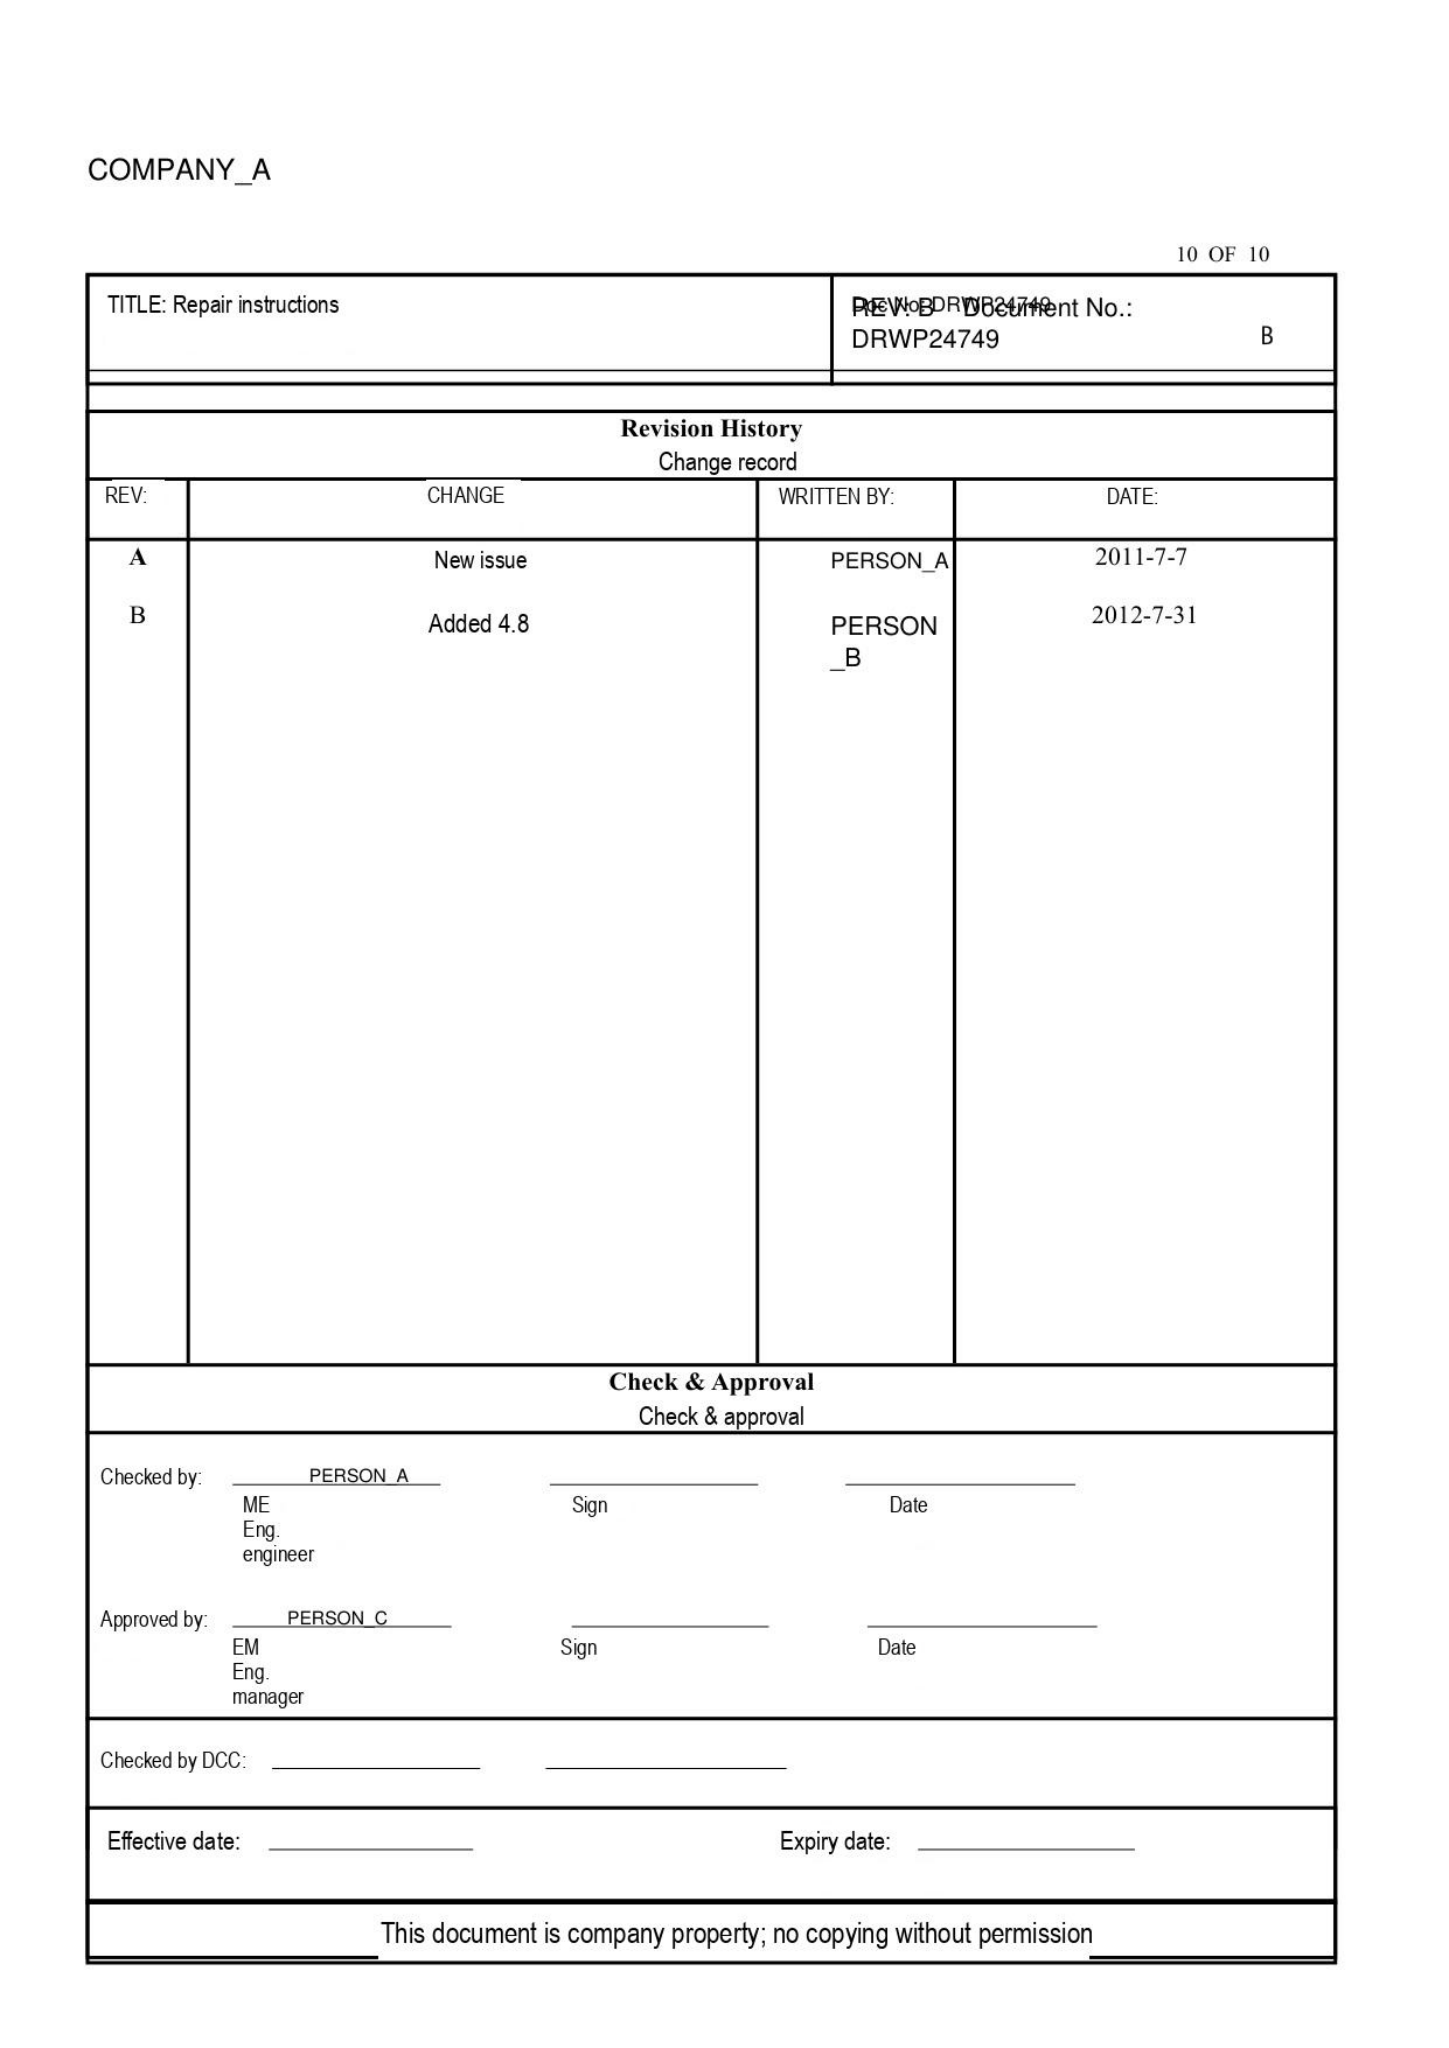COMPANY_A

10 OF 10

| TITLE: Repair instructions | REV: B Document No.: DRWP24749 B |
|---|---|

**Revision History**
Change record

| REV: | CHANGE | WRITTEN BY: | DATE: |
|---|---|---|---|
| A | New issue | PERSON_A | 2011-7-7 |
| B | Added 4.8 | PERSON_B | 2012-7-31 |

**Check & Approval**
Check & approval

Checked by: PERSON_A
ME
Eng.
engineer
Sign
Date

Approved by: PERSON_C
EM
Eng.
manager
Sign
Date

Checked by DCC:

Effective date:
Expiry date:

This document is company property; no copying without permission
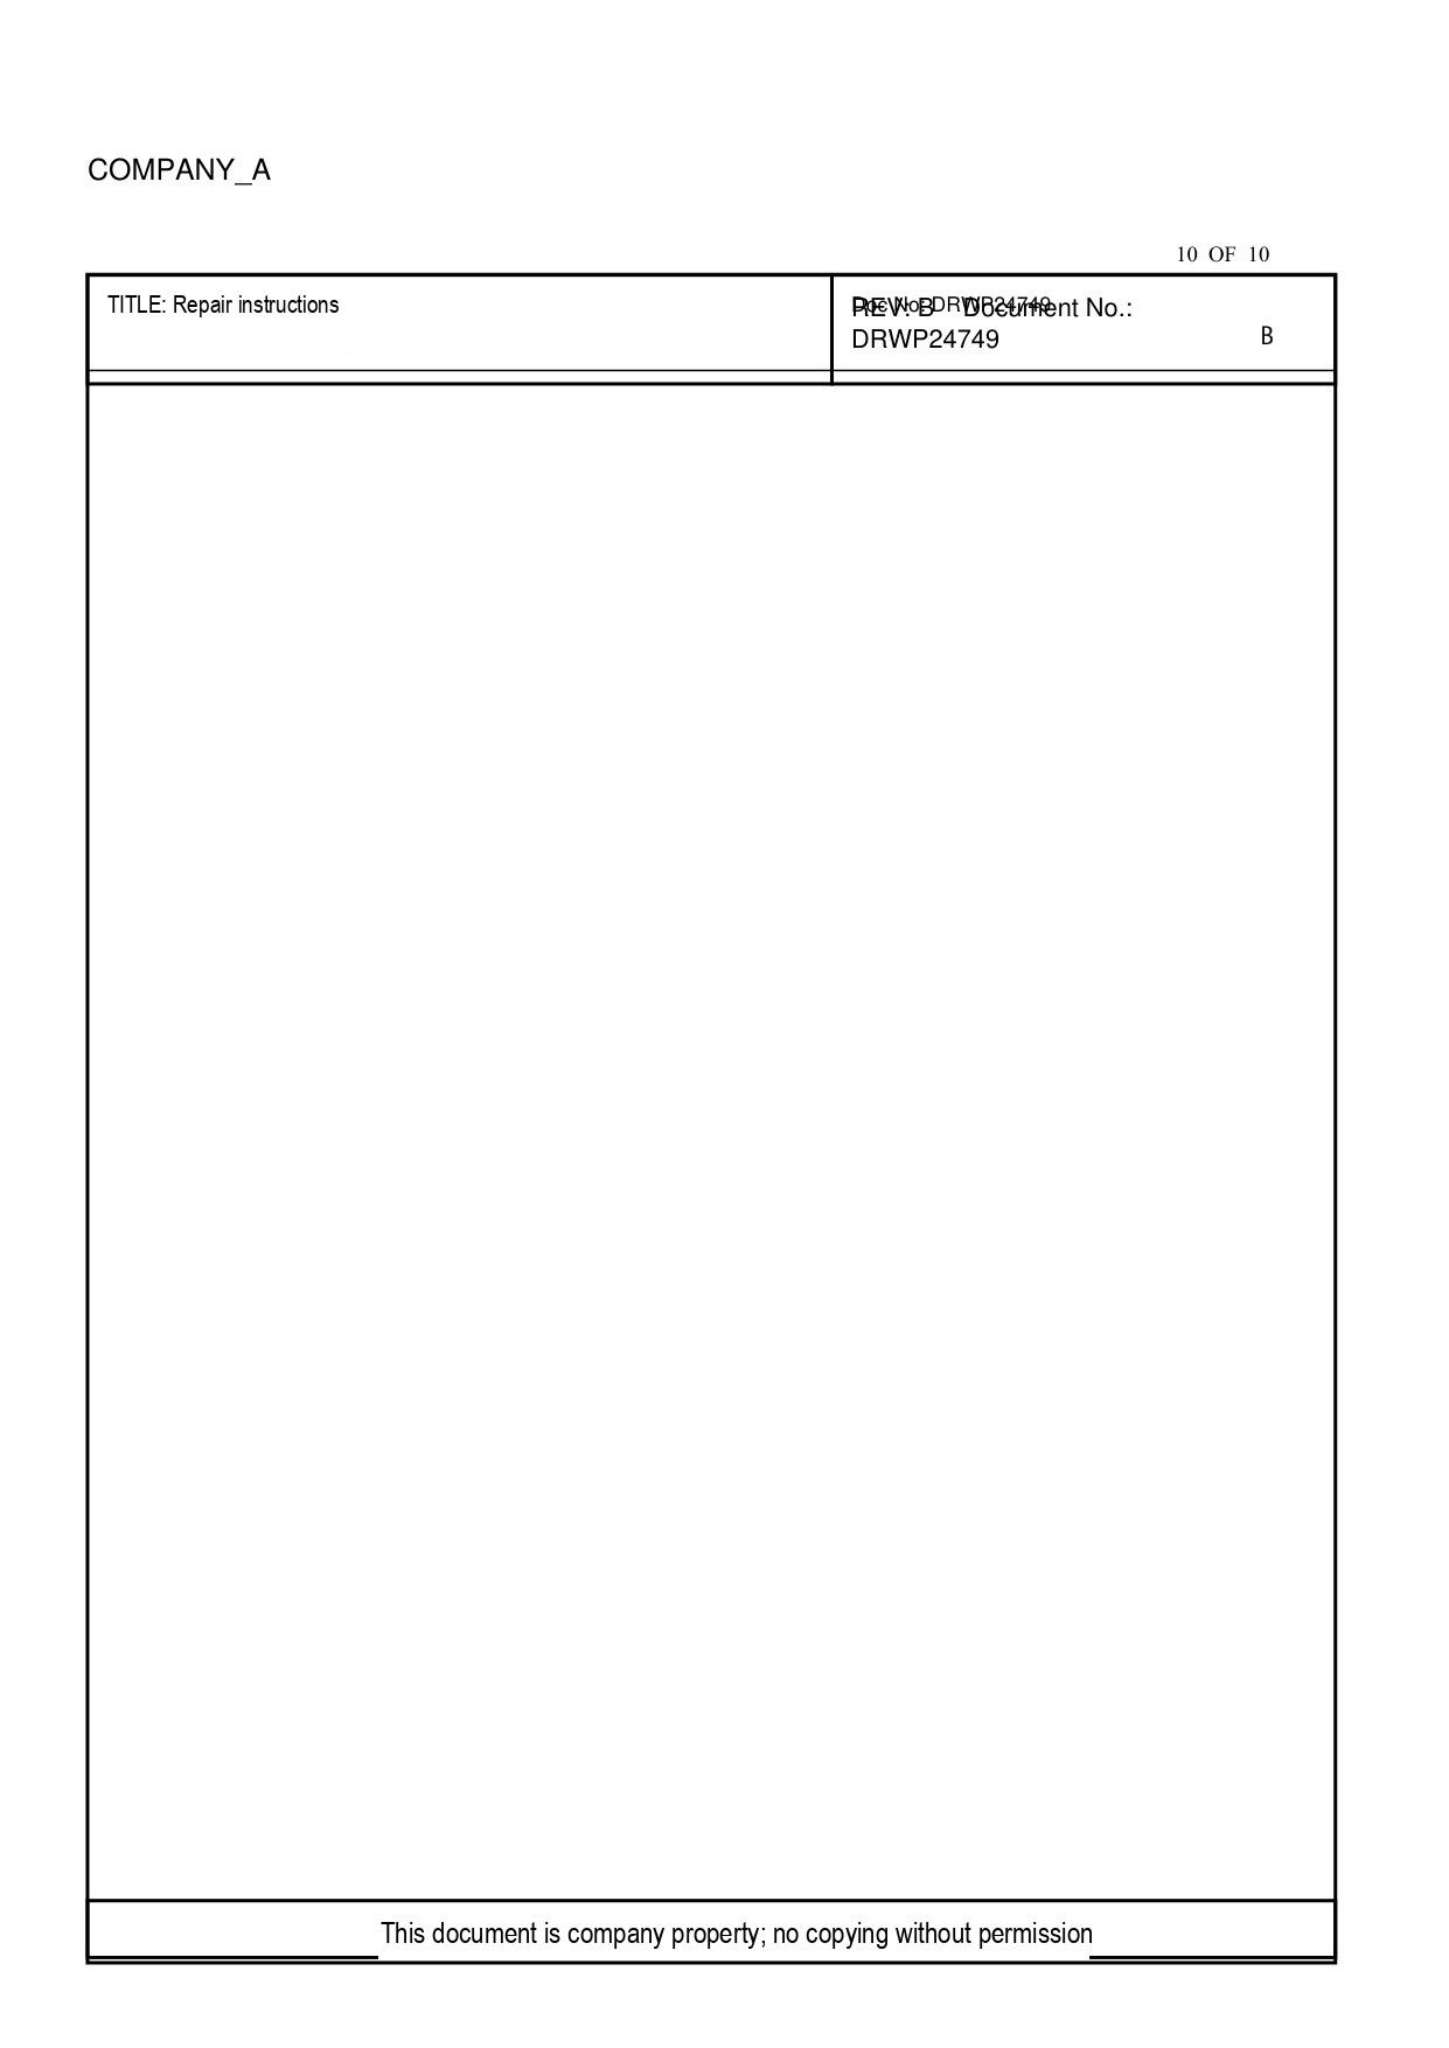COMPANY_A

10 OF 10

| TITLE: Repair instructions | REV: B Document No.: DRWP24749 B |
|---|---|

This document is company property; no copying without permission
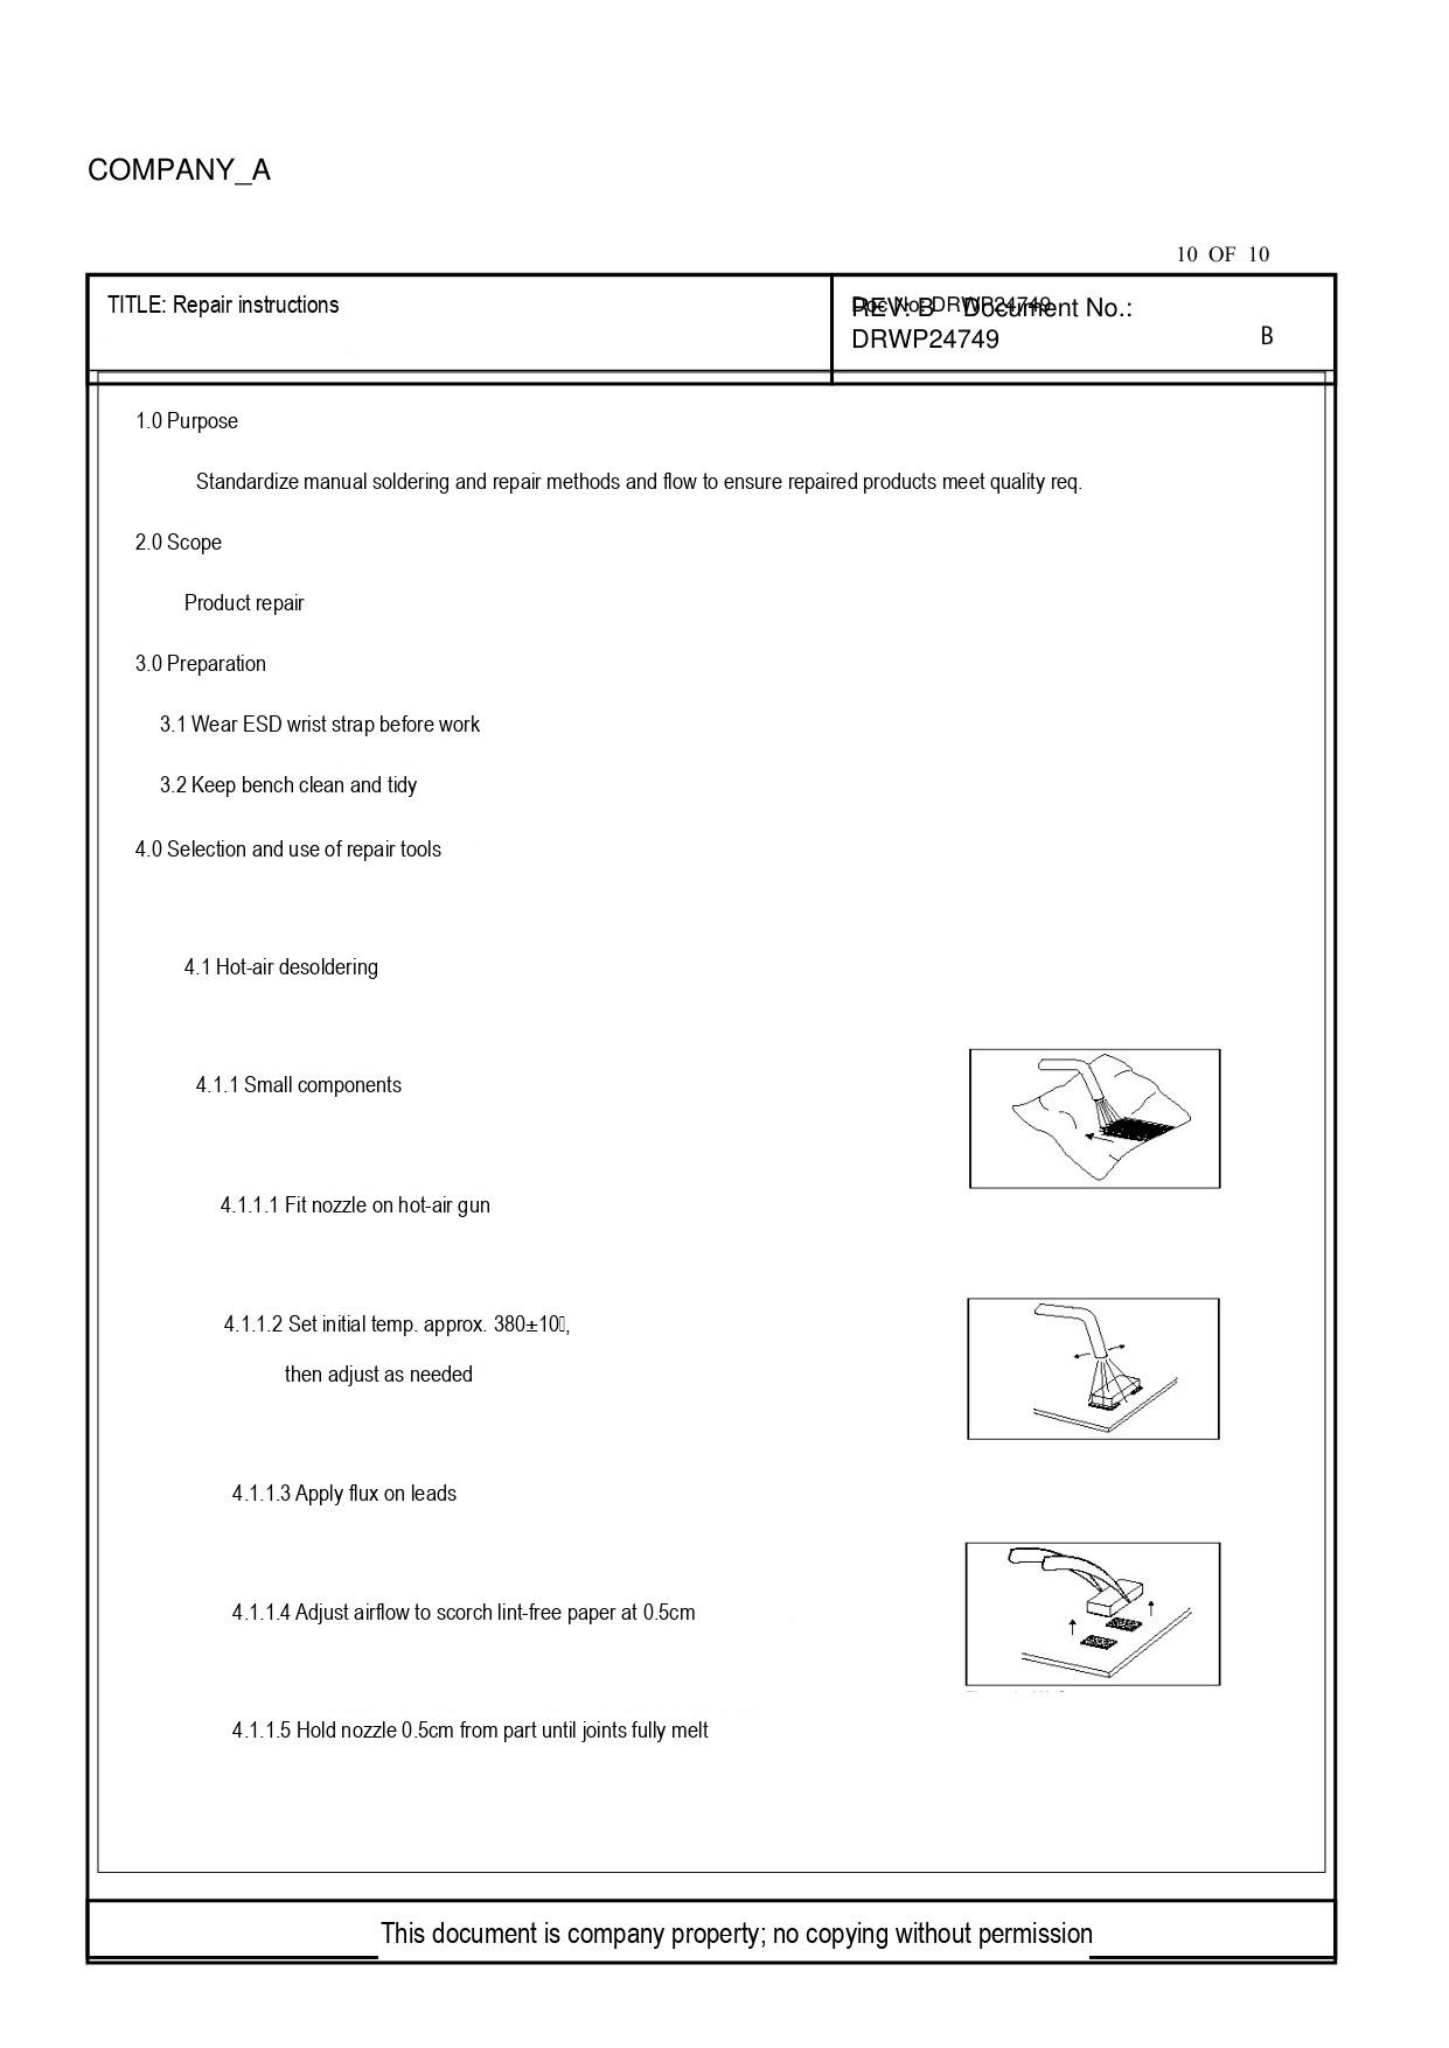COMPANY_A

10 OF 10

| TITLE: Repair instructions | REV: B Document No.: DRWP24749 B |
|---|---|

1.0 Purpose

Standardize manual soldering and repair methods and flow to ensure repaired products meet quality req.

2.0 Scope

Product repair

3.0 Preparation

3.1 Wear ESD wrist strap before work

3.2 Keep bench clean and tidy

4.0 Selection and use of repair tools

4.1 Hot-air desoldering

4.1.1 Small components

4.1.1.1 Fit nozzle on hot-air gun

4.1.1.2 Set initial temp. approx. 380±10,

then adjust as needed

4.1.1.3 Apply flux on leads

4.1.1.4 Adjust airflow to scorch lint-free paper at 0.5cm

4.1.1.5 Hold nozzle 0.5cm from part until joints fully melt

This document is company property; no copying without permission
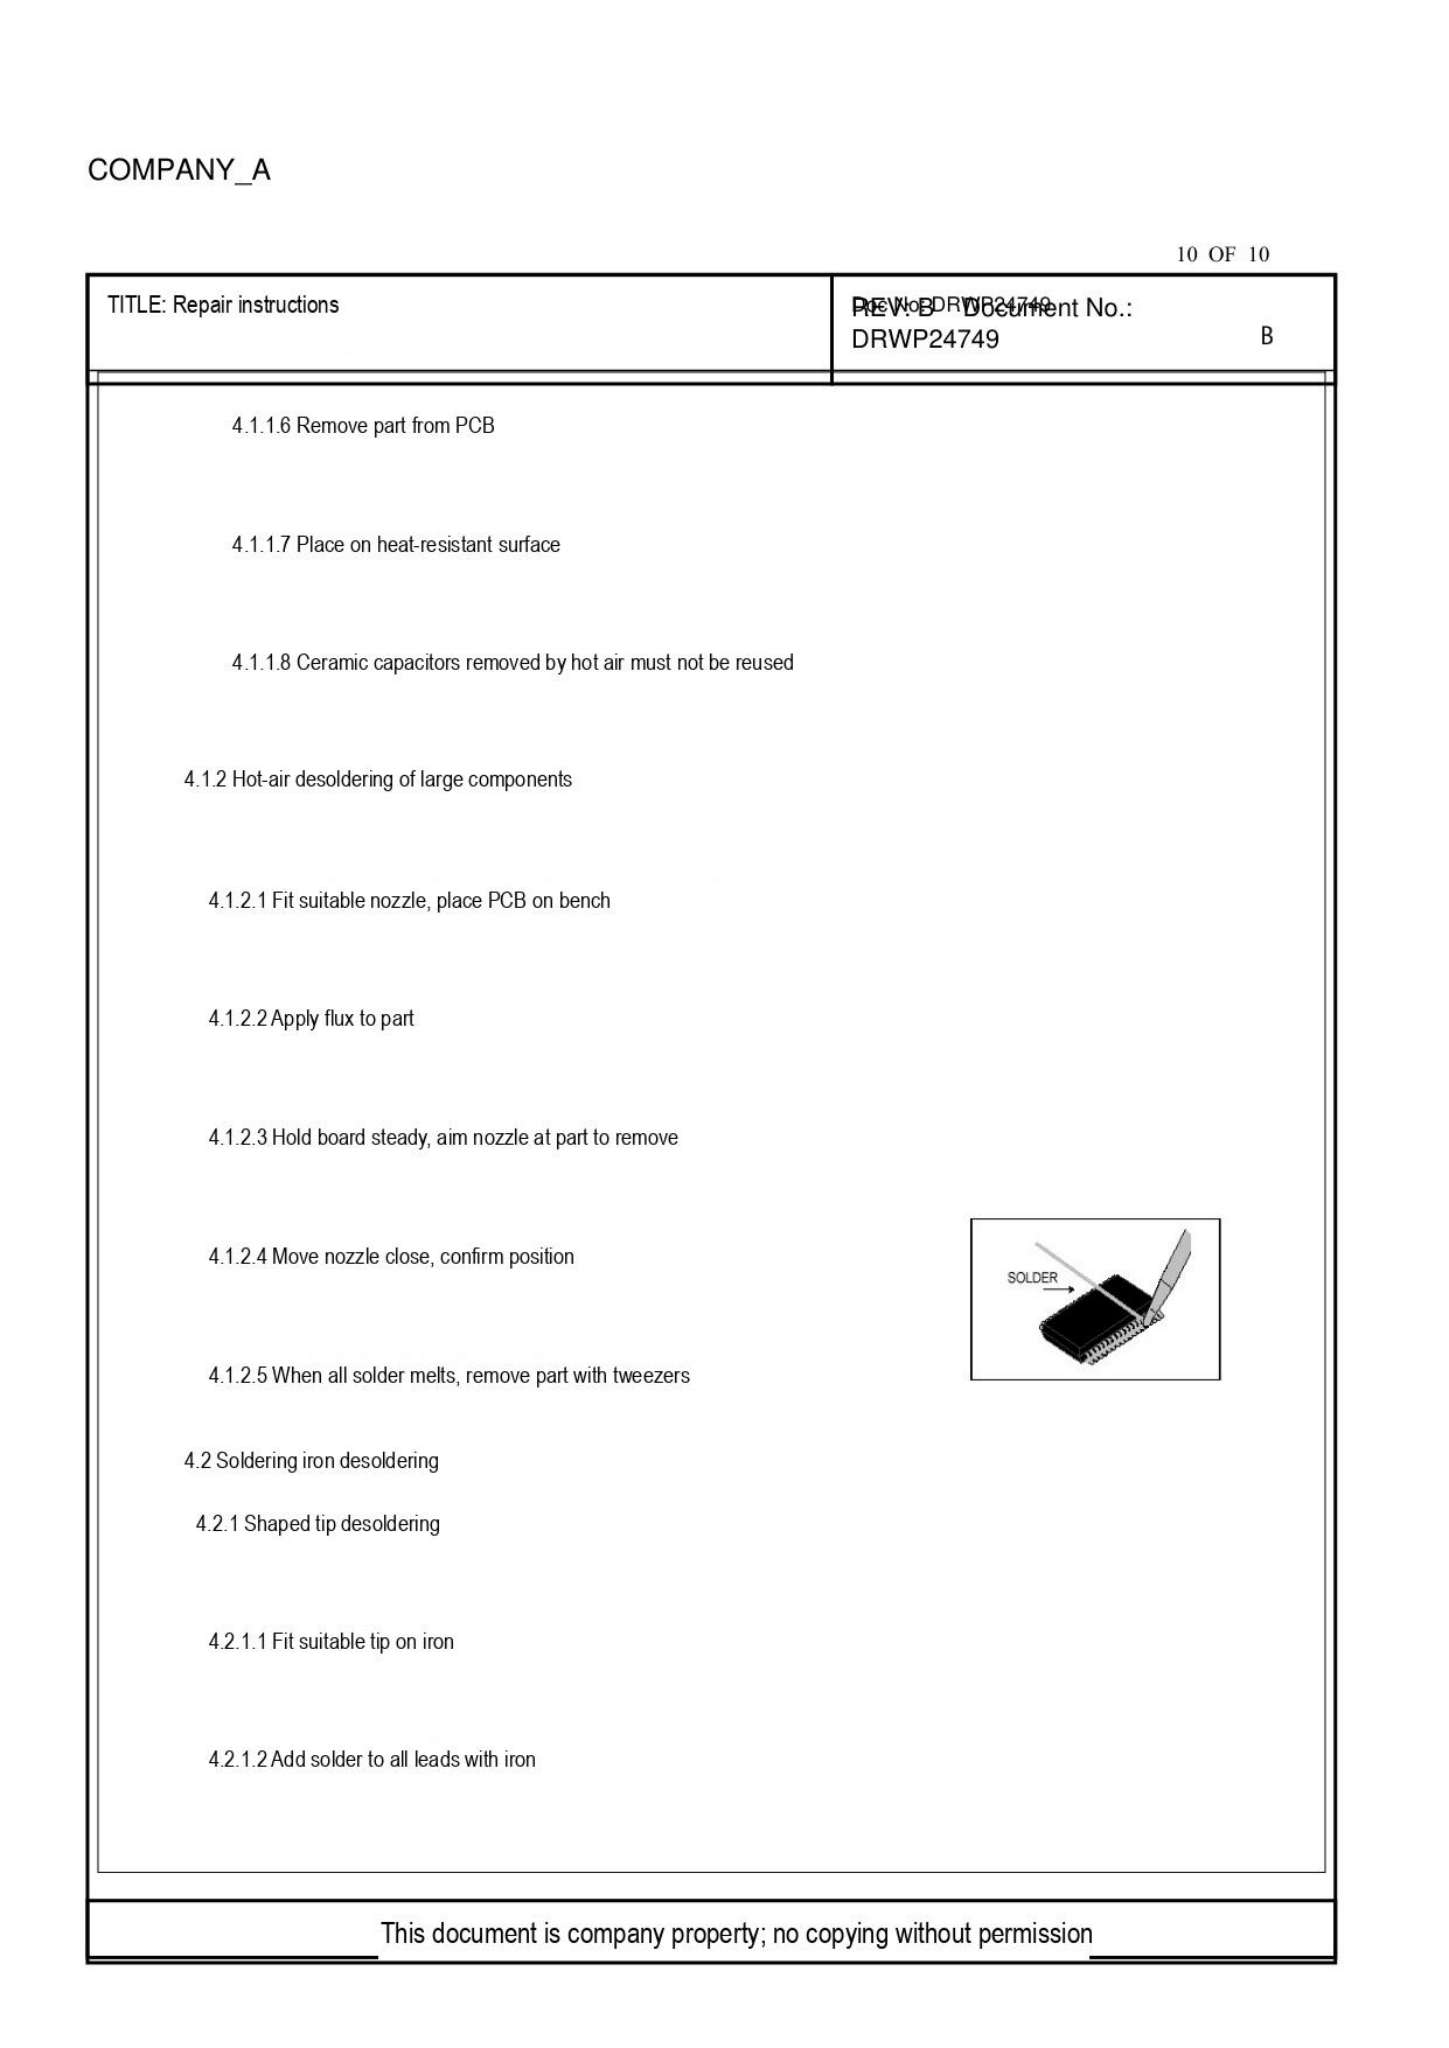COMPANY_A

10 OF 10

| TITLE: Repair instructions | REV: B Document No.: DRWP24749 B |
|---|---|

4.1.1.6 Remove part from PCB

4.1.1.7 Place on heat-resistant surface

4.1.1.8 Ceramic capacitors removed by hot air must not be reused

4.1.2 Hot-air desoldering of large components

4.1.2.1 Fit suitable nozzle, place PCB on bench

4.1.2.2 Apply flux to part

4.1.2.3 Hold board steady, aim nozzle at part to remove

4.1.2.4 Move nozzle close, confirm position

SOLDER

4.1.2.5 When all solder melts, remove part with tweezers

4.2 Soldering iron desoldering

4.2.1 Shaped tip desoldering

4.2.1.1 Fit suitable tip on iron

4.2.1.2 Add solder to all leads with iron

This document is company property; no copying without permission
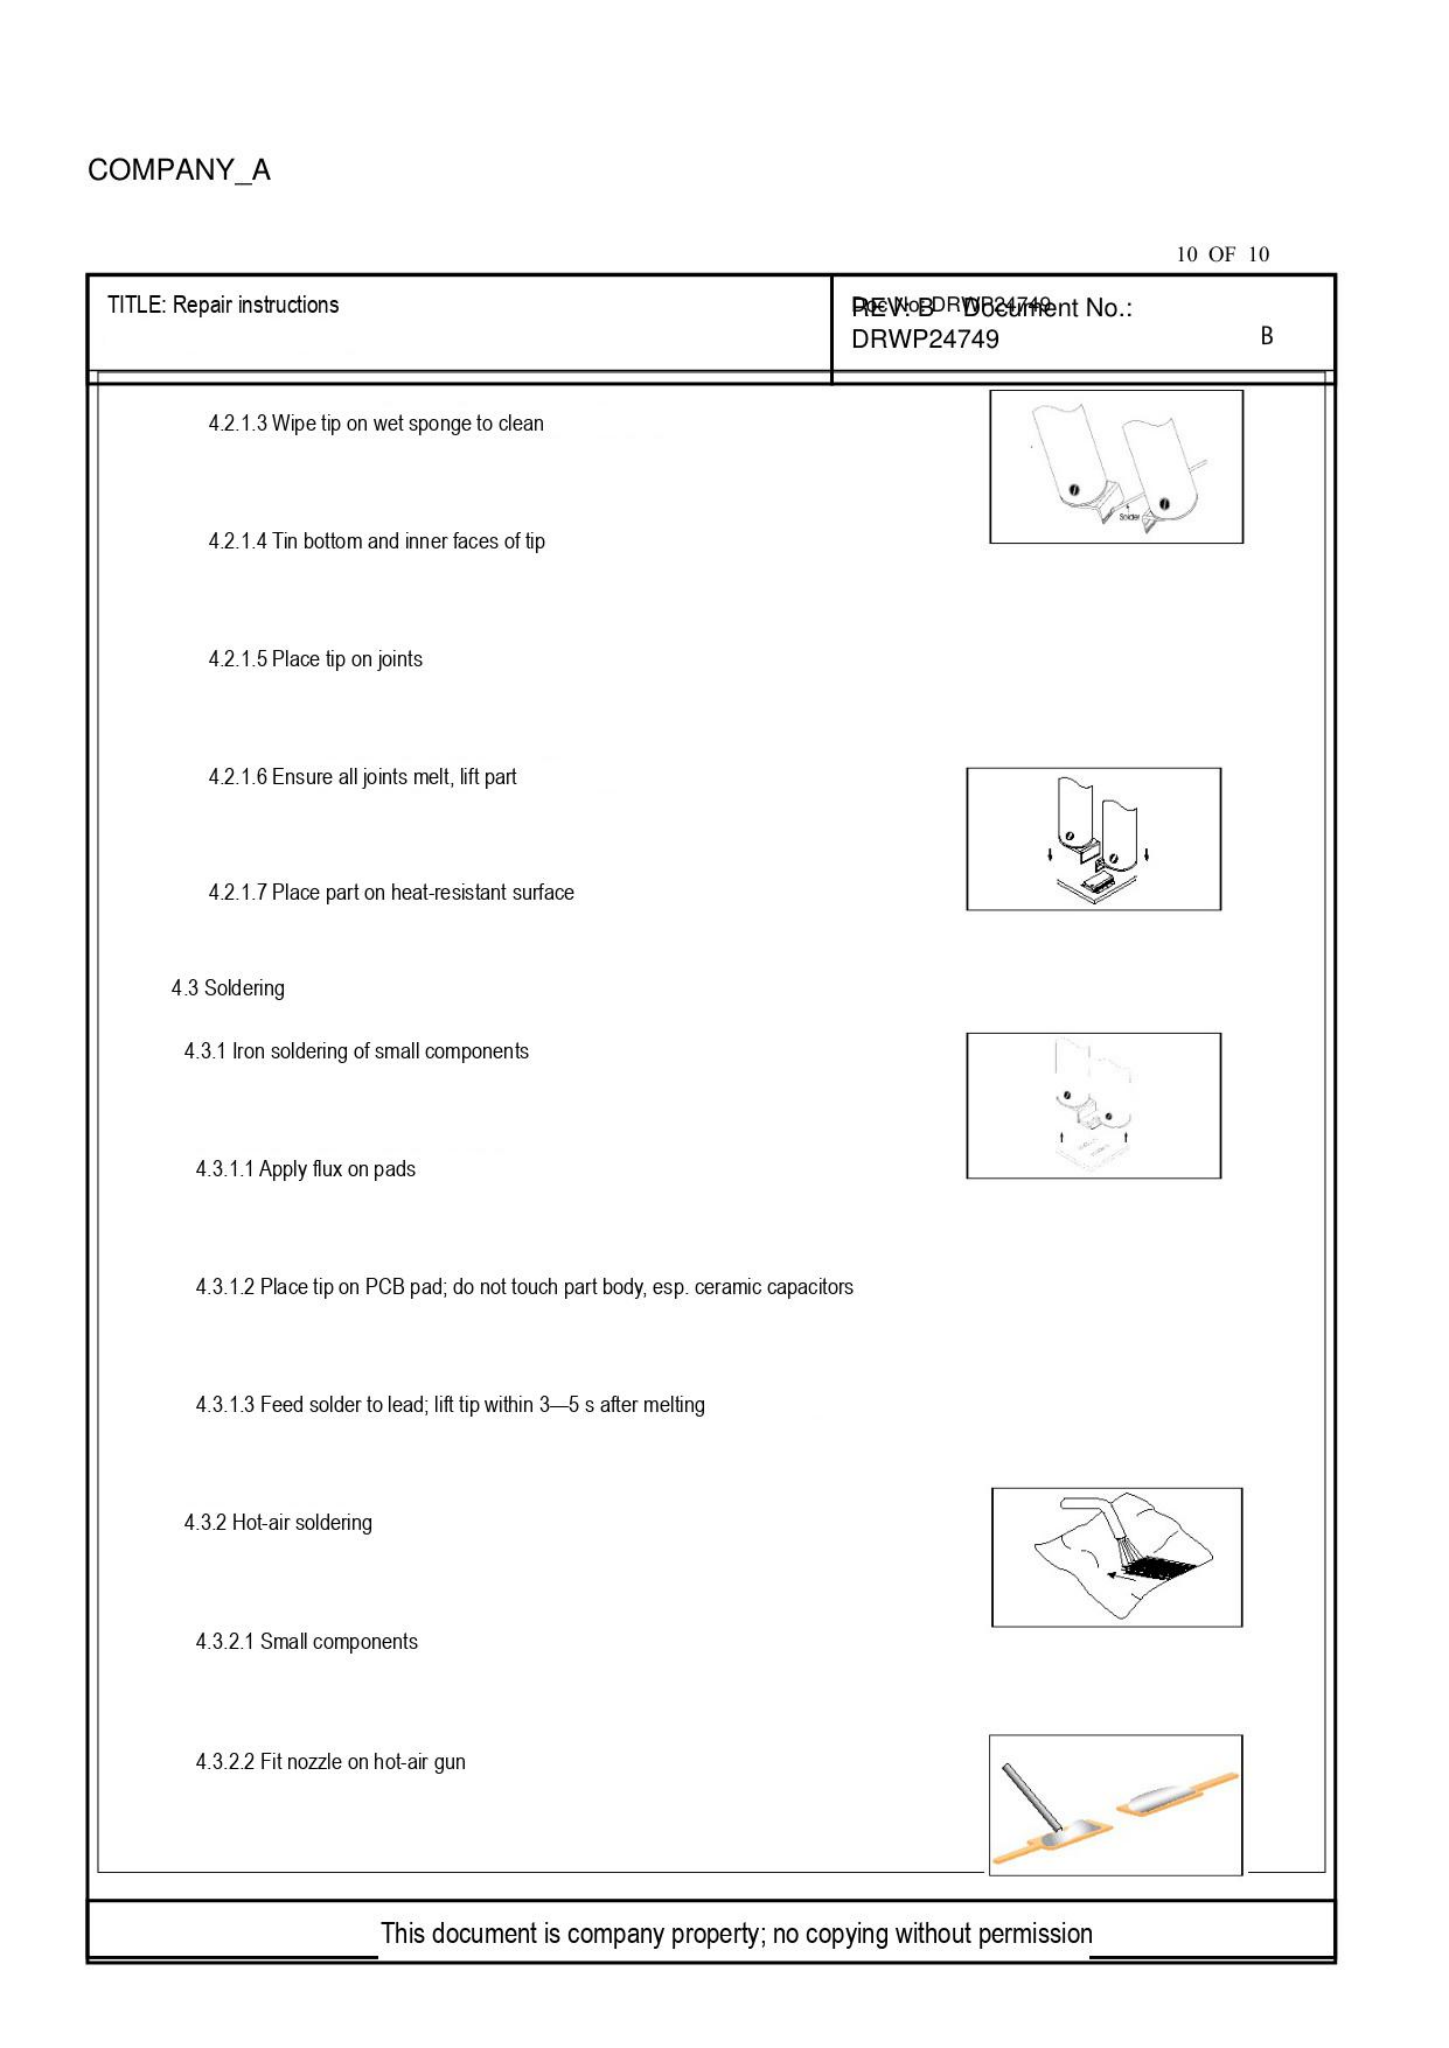COMPANY_A

10 OF 10

| TITLE: Repair instructions | Document No.: DRWP24749 REV: B |
|---|---|

4.2.1.3 Wipe tip on wet sponge to clean

Solder

4.2.1.4 Tin bottom and inner faces of tip

4.2.1.5 Place tip on joints

4.2.1.6 Ensure all joints melt, lift part

4.2.1.7 Place part on heat-resistant surface

4.3 Soldering

4.3.1 Iron soldering of small components

4.3.1.1 Apply flux on pads

4.3.1.2 Place tip on PCB pad; do not touch part body, esp. ceramic capacitors

4.3.1.3 Feed solder to lead; lift tip within 3—5 s after melting

4.3.2 Hot-air soldering

4.3.2.1 Small components

4.3.2.2 Fit nozzle on hot-air gun

This document is company property; no copying without permission
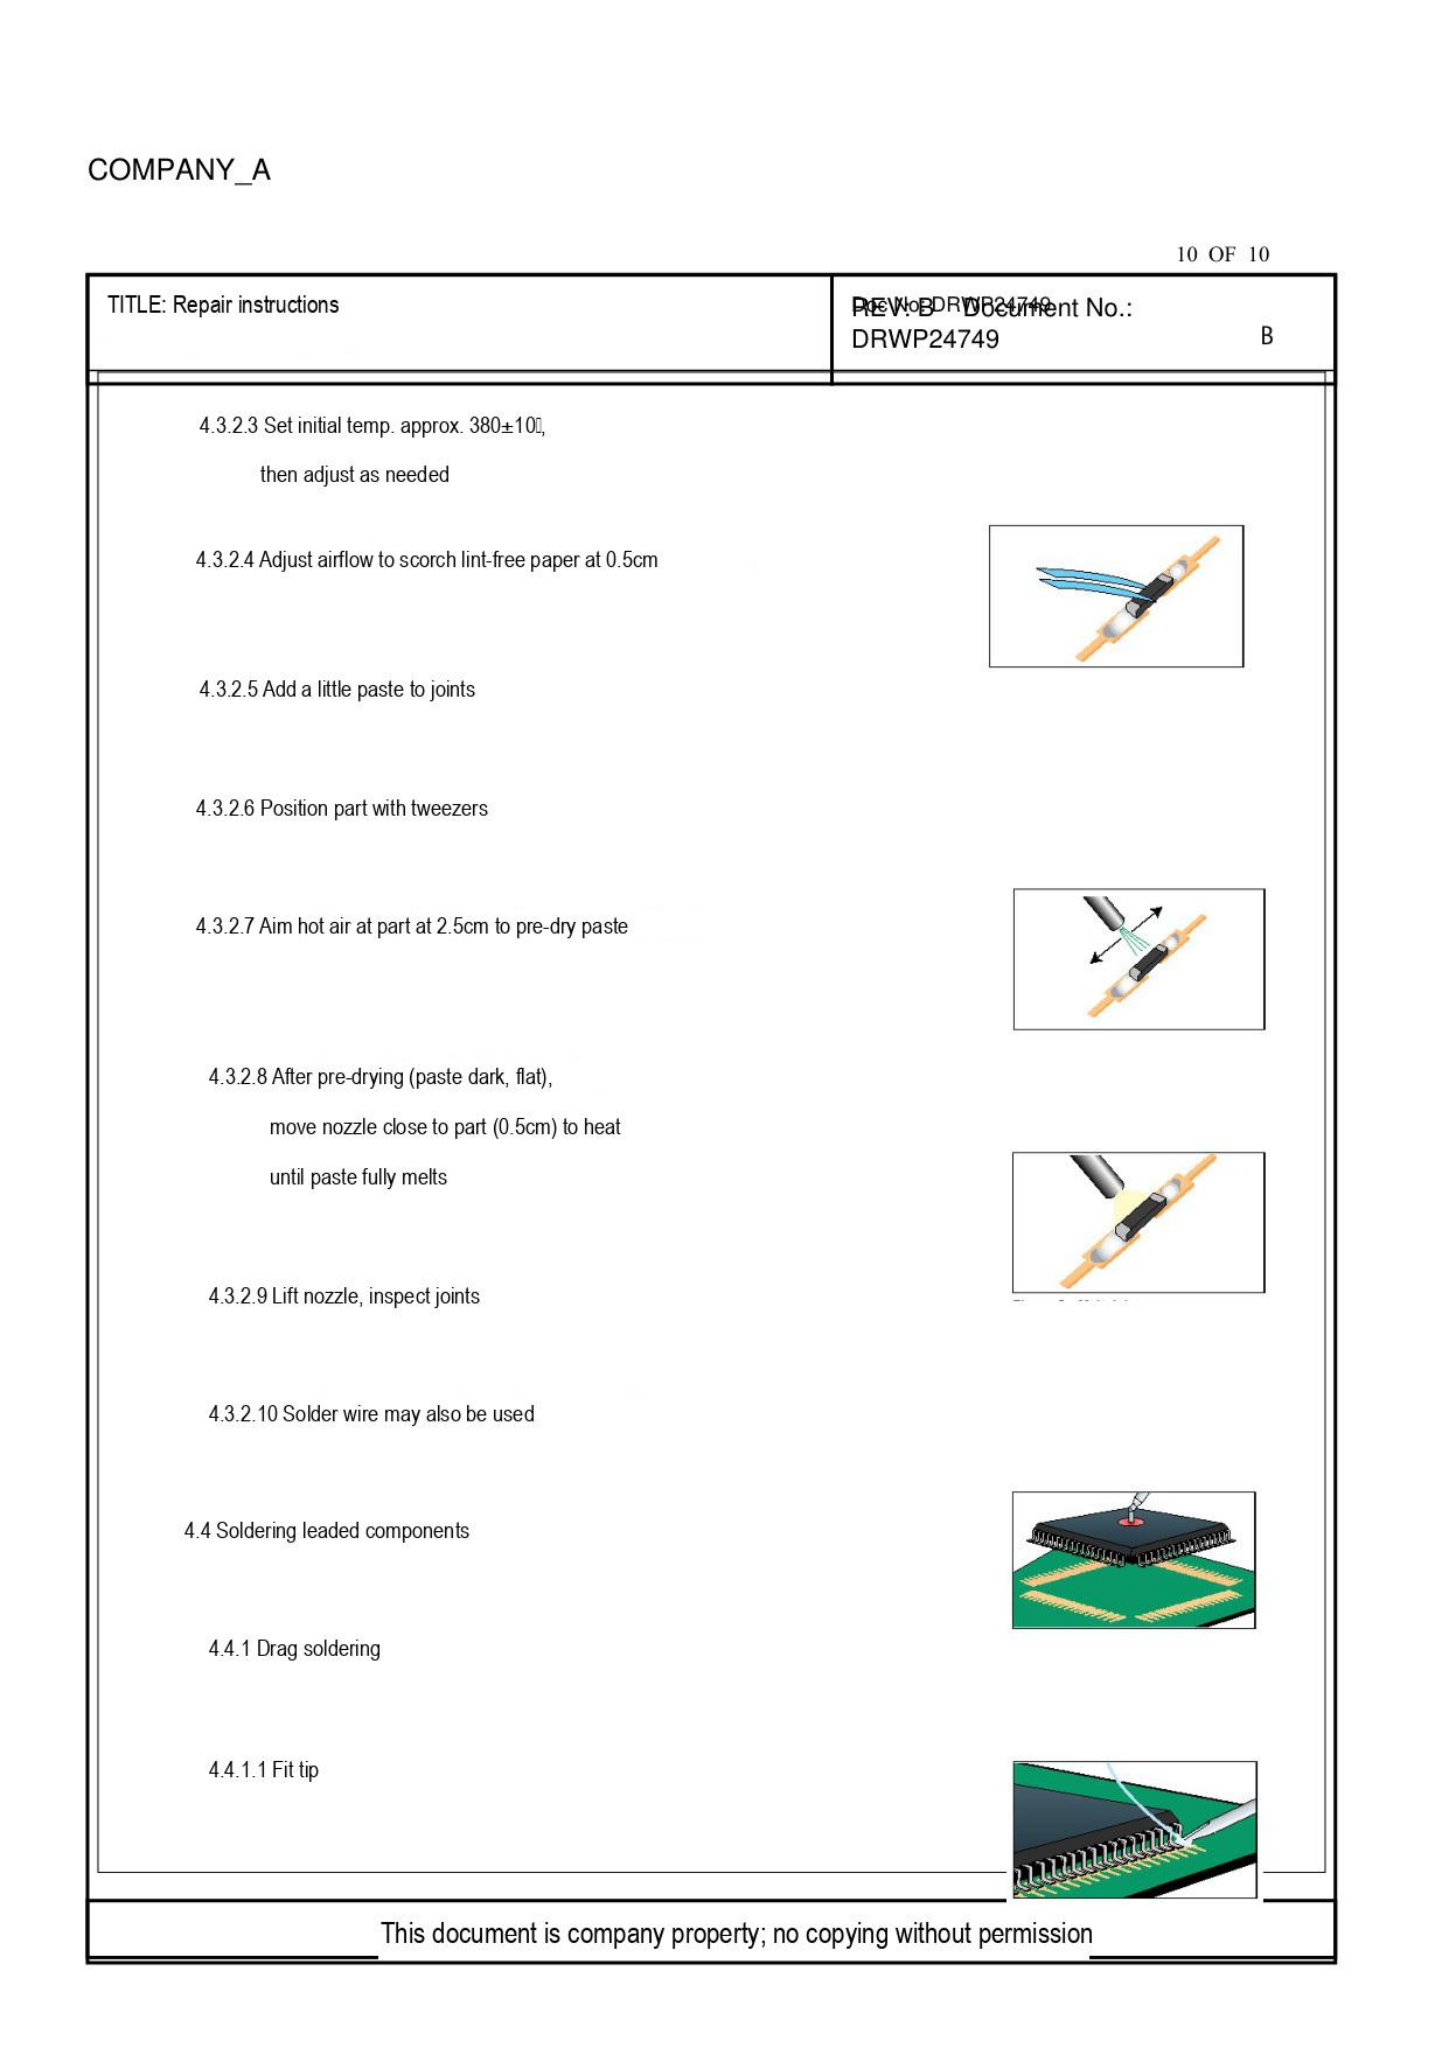COMPANY_A

10 OF 10

| TITLE: Repair instructions | REV: B Document No.: DRWP24749 B |
|---|---|

4.3.2.3 Set initial temp. approx. 380±10,

then adjust as needed

4.3.2.4 Adjust airflow to scorch lint-free paper at 0.5cm

4.3.2.5 Add a little paste to joints

4.3.2.6 Position part with tweezers

4.3.2.7 Aim hot air at part at 2.5cm to pre-dry paste

4.3.2.8 After pre-drying (paste dark, flat),

move nozzle close to part (0.5cm) to heat

until paste fully melts

4.3.2.9 Lift nozzle, inspect joints

4.3.2.10 Solder wire may also be used

4.4 Soldering leaded components

4.4.1 Drag soldering

4.4.1.1 Fit tip

This document is company property; no copying without permission
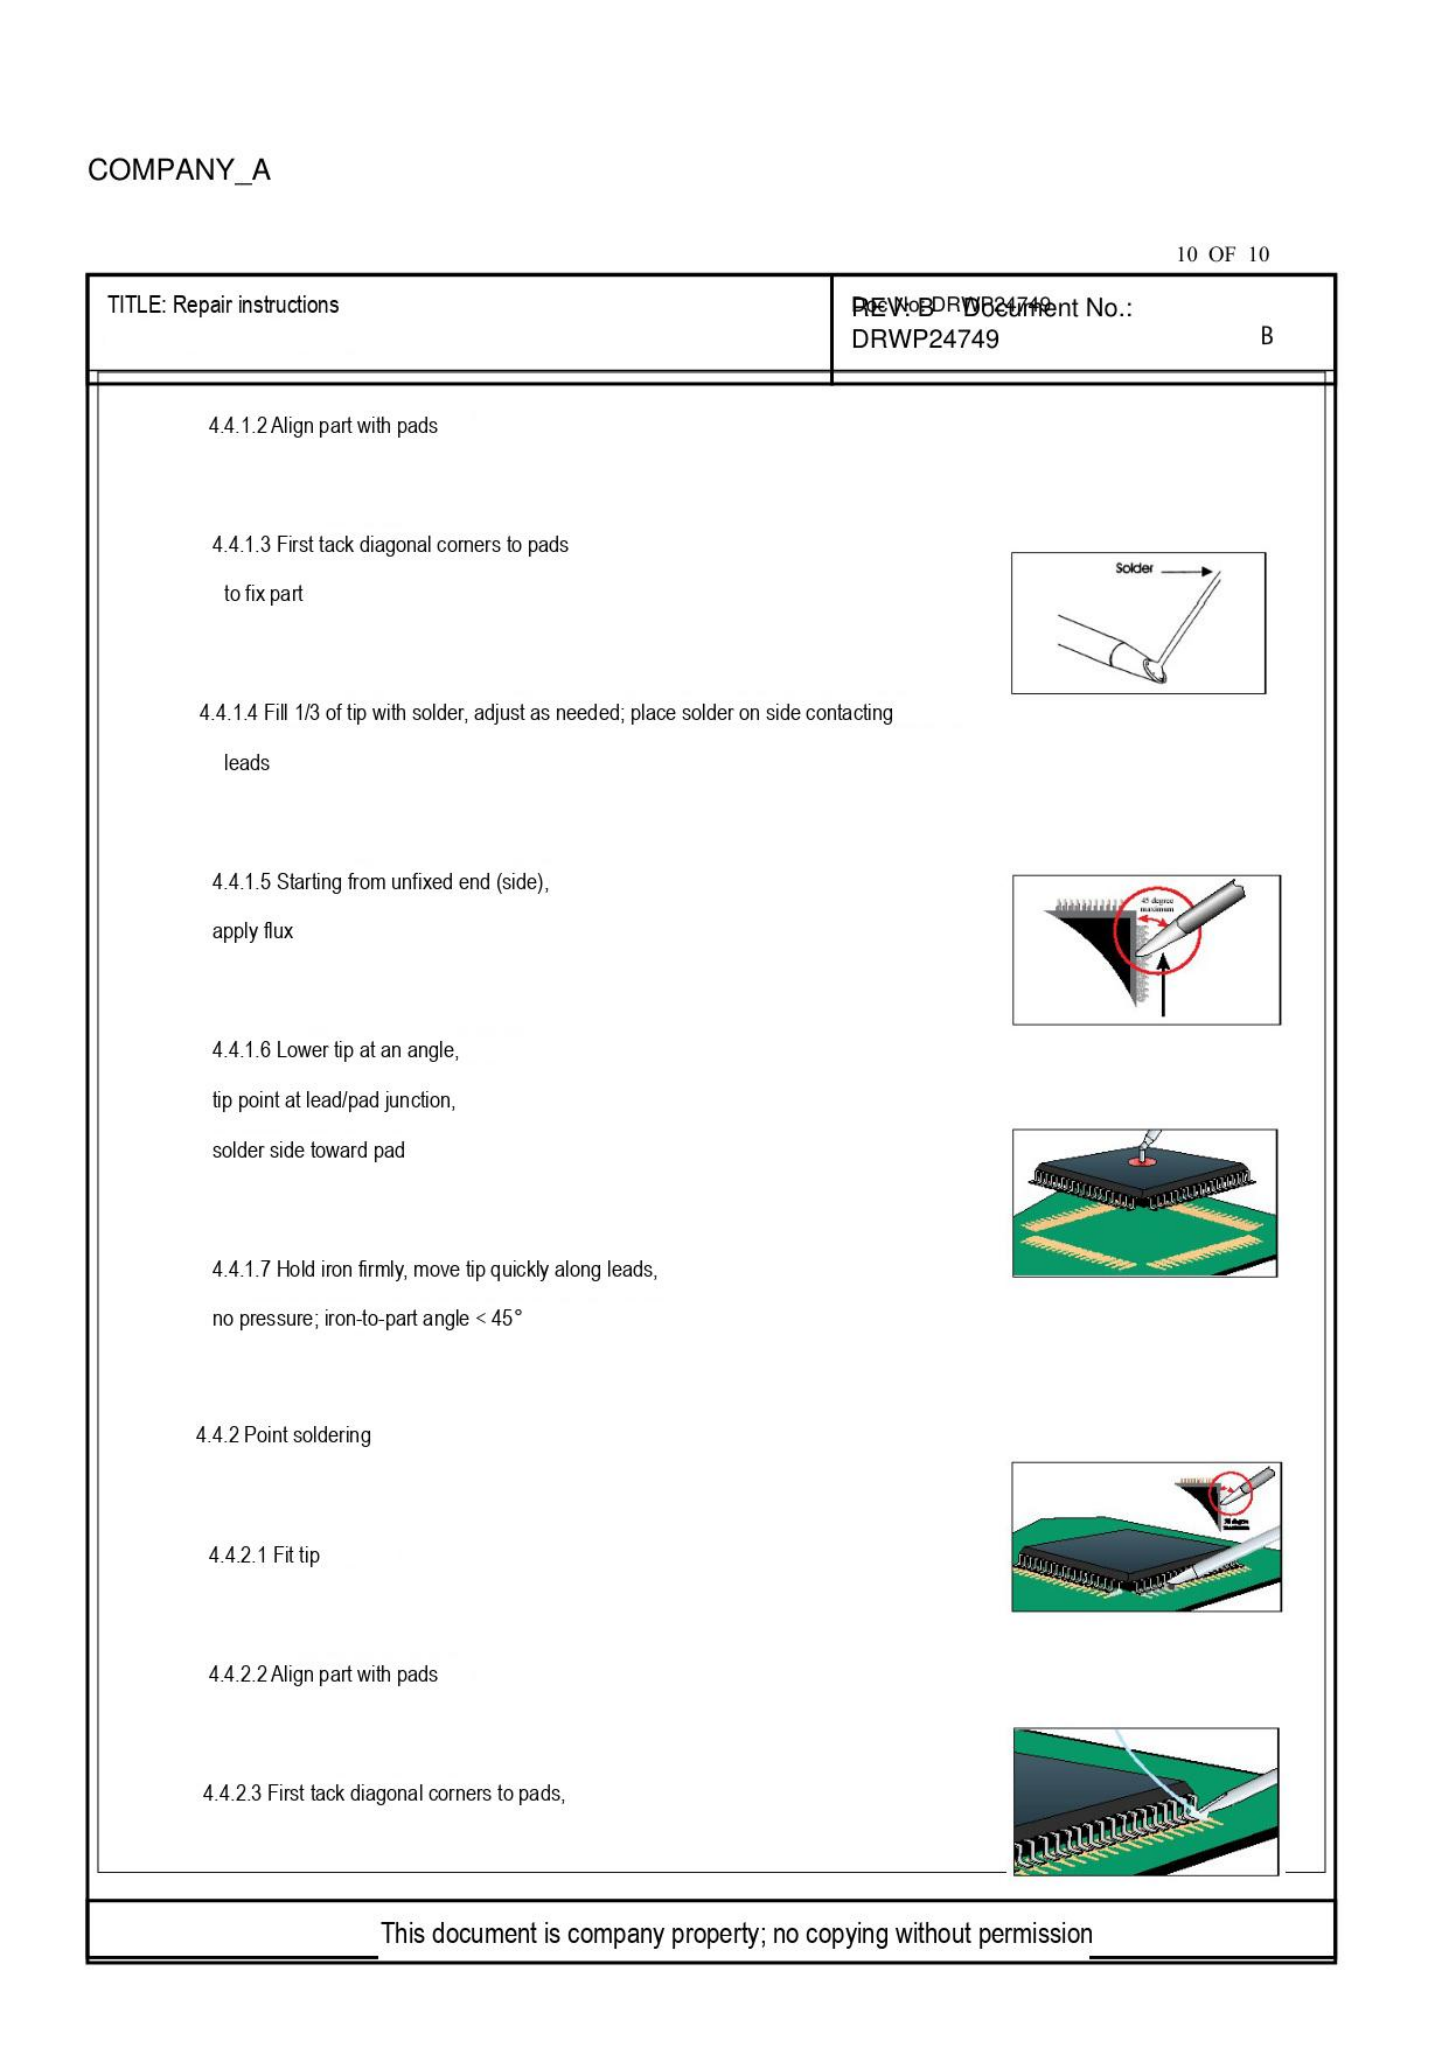COMPANY_A

10 OF 10

| TITLE: Repair instructions | REV: B Document No.: DRWP24749 B |
|---|---|

4.4.1.2 Align part with pads

4.4.1.3 First tack diagonal corners to pads
to fix part

Solder

4.4.1.4 Fill 1/3 of tip with solder, adjust as needed; place solder on side contacting
leads

4.4.1.5 Starting from unfixed end (side),
apply flux

45 degree maximum

4.4.1.6 Lower tip at an angle,
tip point at lead/pad junction,
solder side toward pad

4.4.1.7 Hold iron firmly, move tip quickly along leads,
no pressure; iron-to-part angle < 45°

4.4.2 Point soldering

4.4.2.1 Fit tip

4.4.2.2 Align part with pads

4.4.2.3 First tack diagonal corners to pads,

This document is company property; no copying without permission